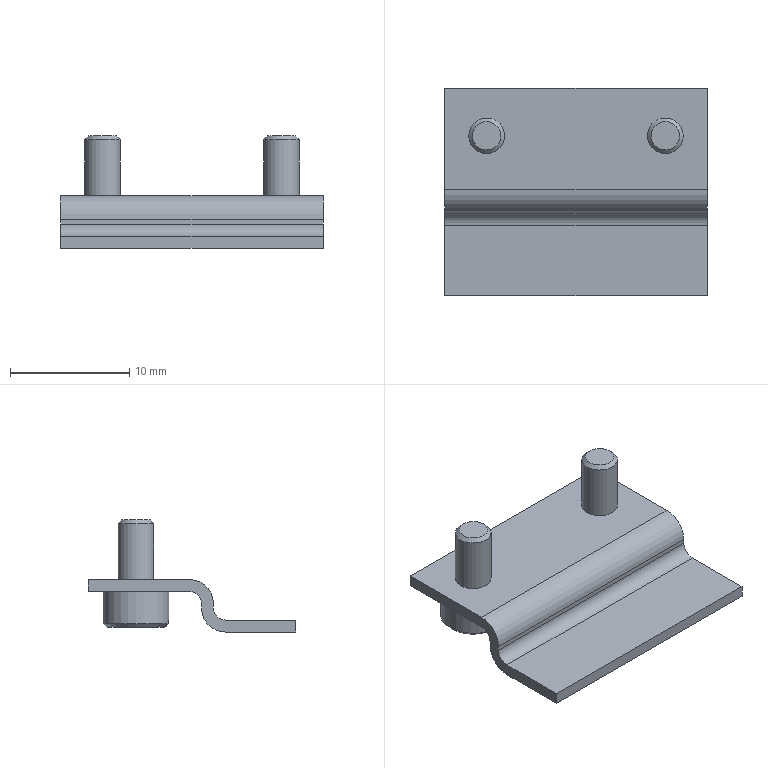Part | STEP file | LX4520CP-MX-B1-590-EP3_f | 1 solid | 40 faces | box 22 x 17.4 x 9.4 mm | volume 629.359 mm3 | plane 28 | cylinder 8 | cone 4 | commonest cylinder face diameters 2 x2 3 x2 4 x2 5.5 x2
STEP:
#1=CARTESIAN_POINT('',(-9.95,0.,-4.));
#2=VERTEX_POINT('',#1);
#3=CARTESIAN_POINT('',(-7.5,0.,-4.));
#4=DIRECTION('',(0.,0.,-1.));
#5=DIRECTION('',(-1.,0.,0.));
#6=AXIS2_PLACEMENT_3D('',#3,#4,#5);
#7=CIRCLE('',#6,2.45);
#8=EDGE_CURVE('',#2,#2,#7,.T.);
#9=ORIENTED_EDGE('',*,*,#8,.T.);
#10=EDGE_LOOP('',(#9));
#11=FACE_OUTER_BOUND('',#10,.T.);
#12=CARTESIAN_POINT('',(-6.25,0.7217,-4.));
#13=VERTEX_POINT('',#12);
#14=CARTESIAN_POINT('',(-7.5,1.443,-4.));
#15=VERTEX_POINT('',#14);
#16=CARTESIAN_POINT('',(-6.25,0.7217,-4.));
#17=DIRECTION('',(-0.866,0.5,0.));
#18=VECTOR('',#17,1000.);
#19=LINE('',#16,#18);
#20=EDGE_CURVE('',#13,#15,#19,.T.);
#21=ORIENTED_EDGE('',*,*,#20,.T.);
#22=CARTESIAN_POINT('',(-8.75,0.7217,-4.));
#23=VERTEX_POINT('',#22);
#24=CARTESIAN_POINT('',(-7.5,1.443,-4.));
#25=DIRECTION('',(-0.866,-0.5,0.));
#26=VECTOR('',#25,1000.);
#27=LINE('',#24,#26);
#28=EDGE_CURVE('',#15,#23,#27,.T.);
#29=ORIENTED_EDGE('',*,*,#28,.T.);
#30=CARTESIAN_POINT('',(-8.75,-0.7217,-4.));
#31=VERTEX_POINT('',#30);
#32=CARTESIAN_POINT('',(-8.75,0.7217,-4.));
#33=DIRECTION('',(0.,-1.,0.));
#34=VECTOR('',#33,1000.);
#35=LINE('',#32,#34);
#36=EDGE_CURVE('',#23,#31,#35,.T.);
#37=ORIENTED_EDGE('',*,*,#36,.T.);
#38=CARTESIAN_POINT('',(-7.5,-1.443,-4.));
#39=VERTEX_POINT('',#38);
#40=CARTESIAN_POINT('',(-8.75,-0.7217,-4.));
#41=DIRECTION('',(0.866,-0.5,0.));
#42=VECTOR('',#41,1000.);
#43=LINE('',#40,#42);
#44=EDGE_CURVE('',#31,#39,#43,.T.);
#45=ORIENTED_EDGE('',*,*,#44,.T.);
#46=CARTESIAN_POINT('',(-6.25,-0.7217,-4.));
#47=VERTEX_POINT('',#46);
#48=CARTESIAN_POINT('',(-7.5,-1.443,-4.));
#49=DIRECTION('',(0.866,0.5,0.));
#50=VECTOR('',#49,1000.);
#51=LINE('',#48,#50);
#52=EDGE_CURVE('',#39,#47,#51,.T.);
#53=ORIENTED_EDGE('',*,*,#52,.T.);
#54=CARTESIAN_POINT('',(-6.25,-0.7217,-4.));
#55=DIRECTION('',(0.,1.,0.));
#56=VECTOR('',#55,1000.);
#57=LINE('',#54,#56);
#58=EDGE_CURVE('',#47,#13,#57,.T.);
#59=ORIENTED_EDGE('',*,*,#58,.T.);
#60=EDGE_LOOP('',(#21,#29,#37,#45,#53,#59));
#61=FACE_BOUND('',#60,.T.);
#62=CARTESIAN_POINT('',(-7.5,2.45,-4.));
#63=DIRECTION('',(0.,0.,1.));
#64=DIRECTION('',(1.,0.,0.));
#65=AXIS2_PLACEMENT_3D('',#62,#63,#64);
#66=PLANE('',#65);
#67=ADVANCED_FACE('',(#11,#61),#66,.F.);
#68=CARTESIAN_POINT('',(5.05,0.,-4.));
#69=VERTEX_POINT('',#68);
#70=CARTESIAN_POINT('',(7.5,0.,-4.));
#71=DIRECTION('',(0.,0.,-1.));
#72=DIRECTION('',(-1.,0.,0.));
#73=AXIS2_PLACEMENT_3D('',#70,#71,#72);
#74=CIRCLE('',#73,2.45);
#75=EDGE_CURVE('',#69,#69,#74,.T.);
#76=ORIENTED_EDGE('',*,*,#75,.T.);
#77=EDGE_LOOP('',(#76));
#78=FACE_OUTER_BOUND('',#77,.T.);
#79=CARTESIAN_POINT('',(8.75,0.7217,-4.));
#80=VERTEX_POINT('',#79);
#81=CARTESIAN_POINT('',(7.5,1.443,-4.));
#82=VERTEX_POINT('',#81);
#83=CARTESIAN_POINT('',(8.75,0.7217,-4.));
#84=DIRECTION('',(-0.866,0.5,0.));
#85=VECTOR('',#84,1000.);
#86=LINE('',#83,#85);
#87=EDGE_CURVE('',#80,#82,#86,.T.);
#88=ORIENTED_EDGE('',*,*,#87,.T.);
#89=CARTESIAN_POINT('',(6.25,0.7217,-4.));
#90=VERTEX_POINT('',#89);
#91=CARTESIAN_POINT('',(7.5,1.443,-4.));
#92=DIRECTION('',(-0.866,-0.5,0.));
#93=VECTOR('',#92,1000.);
#94=LINE('',#91,#93);
#95=EDGE_CURVE('',#82,#90,#94,.T.);
#96=ORIENTED_EDGE('',*,*,#95,.T.);
#97=CARTESIAN_POINT('',(6.25,-0.7217,-4.));
#98=VERTEX_POINT('',#97);
#99=CARTESIAN_POINT('',(6.25,0.7217,-4.));
#100=DIRECTION('',(0.,-1.,0.));
#101=VECTOR('',#100,1000.);
#102=LINE('',#99,#101);
#103=EDGE_CURVE('',#90,#98,#102,.T.);
#104=ORIENTED_EDGE('',*,*,#103,.T.);
#105=CARTESIAN_POINT('',(7.5,-1.443,-4.));
#106=VERTEX_POINT('',#105);
#107=CARTESIAN_POINT('',(6.25,-0.7217,-4.));
#108=DIRECTION('',(0.866,-0.5,0.));
#109=VECTOR('',#108,1000.);
#110=LINE('',#107,#109);
#111=EDGE_CURVE('',#98,#106,#110,.T.);
#112=ORIENTED_EDGE('',*,*,#111,.T.);
#113=CARTESIAN_POINT('',(8.75,-0.7217,-4.));
#114=VERTEX_POINT('',#113);
#115=CARTESIAN_POINT('',(7.5,-1.443,-4.));
#116=DIRECTION('',(0.866,0.5,0.));
#117=VECTOR('',#116,1000.);
#118=LINE('',#115,#117);
#119=EDGE_CURVE('',#106,#114,#118,.T.);
#120=ORIENTED_EDGE('',*,*,#119,.T.);
#121=CARTESIAN_POINT('',(8.75,-0.7217,-4.));
#122=DIRECTION('',(0.,1.,0.));
#123=VECTOR('',#122,1000.);
#124=LINE('',#121,#123);
#125=EDGE_CURVE('',#114,#80,#124,.T.);
#126=ORIENTED_EDGE('',*,*,#125,.T.);
#127=EDGE_LOOP('',(#88,#96,#104,#112,#120,#126));
#128=FACE_BOUND('',#127,.T.);
#129=CARTESIAN_POINT('',(7.5,2.45,-4.));
#130=DIRECTION('',(0.,0.,1.));
#131=DIRECTION('',(1.,0.,0.));
#132=AXIS2_PLACEMENT_3D('',#129,#130,#131);
#133=PLANE('',#132);
#134=ADVANCED_FACE('',(#78,#128),#133,.F.);
#135=CARTESIAN_POINT('',(-11.,4.,-1.));
#136=VERTEX_POINT('',#135);
#137=CARTESIAN_POINT('',(-11.,4.,0.));
#138=VERTEX_POINT('',#137);
#139=CARTESIAN_POINT('',(-11.,4.,-1.));
#140=DIRECTION('',(0.,0.,1.));
#141=VECTOR('',#140,1000.);
#142=LINE('',#139,#141);
#143=EDGE_CURVE('',#136,#138,#142,.T.);
#144=ORIENTED_EDGE('',*,*,#143,.T.);
#145=CARTESIAN_POINT('',(11.,4.,0.));
#146=VERTEX_POINT('',#145);
#147=CARTESIAN_POINT('',(11.,4.,0.));
#148=DIRECTION('',(-1.,0.,0.));
#149=VECTOR('',#148,1000.);
#150=LINE('',#147,#149);
#151=EDGE_CURVE('',#146,#138,#150,.T.);
#152=ORIENTED_EDGE('',*,*,#151,.F.);
#153=CARTESIAN_POINT('',(11.,4.,-1.));
#154=VERTEX_POINT('',#153);
#155=CARTESIAN_POINT('',(11.,4.,-1.));
#156=DIRECTION('',(0.,0.,1.));
#157=VECTOR('',#156,1000.);
#158=LINE('',#155,#157);
#159=EDGE_CURVE('',#154,#146,#158,.T.);
#160=ORIENTED_EDGE('',*,*,#159,.F.);
#161=CARTESIAN_POINT('',(11.,4.,-1.));
#162=DIRECTION('',(-1.,0.,0.));
#163=VECTOR('',#162,1000.);
#164=LINE('',#161,#163);
#165=EDGE_CURVE('',#154,#136,#164,.T.);
#166=ORIENTED_EDGE('',*,*,#165,.T.);
#167=EDGE_LOOP('',(#144,#152,#160,#166));
#168=FACE_OUTER_BOUND('',#167,.T.);
#169=CARTESIAN_POINT('',(11.,4.,-1.));
#170=DIRECTION('',(0.,-1.,0.));
#171=DIRECTION('',(0.,0.,-1.));
#172=AXIS2_PLACEMENT_3D('',#169,#170,#171);
#173=PLANE('',#172);
#174=ADVANCED_FACE('',(#168),#173,.F.);
#175=CARTESIAN_POINT('',(-11.,-4.5,0.));
#176=VERTEX_POINT('',#175);
#177=CARTESIAN_POINT('',(-11.,4.,0.));
#178=DIRECTION('',(0.,-1.,0.));
#179=VECTOR('',#178,1000.);
#180=LINE('',#177,#179);
#181=EDGE_CURVE('',#138,#176,#180,.T.);
#182=ORIENTED_EDGE('',*,*,#181,.T.);
#183=CARTESIAN_POINT('',(11.,-4.5,0.));
#184=VERTEX_POINT('',#183);
#185=CARTESIAN_POINT('',(11.,-4.5,0.));
#186=DIRECTION('',(-1.,0.,0.));
#187=VECTOR('',#186,1000.);
#188=LINE('',#185,#187);
#189=EDGE_CURVE('',#184,#176,#188,.T.);
#190=ORIENTED_EDGE('',*,*,#189,.F.);
#191=CARTESIAN_POINT('',(11.,4.,0.));
#192=DIRECTION('',(0.,-1.,0.));
#193=VECTOR('',#192,1000.);
#194=LINE('',#191,#193);
#195=EDGE_CURVE('',#146,#184,#194,.T.);
#196=ORIENTED_EDGE('',*,*,#195,.F.);
#197=ORIENTED_EDGE('',*,*,#151,.T.);
#198=EDGE_LOOP('',(#182,#190,#196,#197));
#199=FACE_OUTER_BOUND('',#198,.T.);
#200=CARTESIAN_POINT('',(-9.,0.,0.));
#201=VERTEX_POINT('',#200);
#202=CARTESIAN_POINT('',(-6.,0.,0.));
#203=VERTEX_POINT('',#202);
#204=CARTESIAN_POINT('',(-7.5,0.,0.));
#205=DIRECTION('',(0.,0.,-1.));
#206=DIRECTION('',(-1.,0.,0.));
#207=AXIS2_PLACEMENT_3D('',#204,#205,#206);
#208=CIRCLE('',#207,1.5);
#209=EDGE_CURVE('',#201,#203,#208,.F.);
#210=ORIENTED_EDGE('',*,*,#209,.F.);
#211=CARTESIAN_POINT('',(-7.5,0.,0.));
#212=DIRECTION('',(0.,0.,-1.));
#213=DIRECTION('',(-1.,0.,0.));
#214=AXIS2_PLACEMENT_3D('',#211,#212,#213);
#215=CIRCLE('',#214,1.5);
#216=EDGE_CURVE('',#203,#201,#215,.F.);
#217=ORIENTED_EDGE('',*,*,#216,.F.);
#218=EDGE_LOOP('',(#210,#217));
#219=FACE_BOUND('',#218,.T.);
#220=CARTESIAN_POINT('',(6.,0.,0.));
#221=VERTEX_POINT('',#220);
#222=CARTESIAN_POINT('',(9.,0.,0.));
#223=VERTEX_POINT('',#222);
#224=CARTESIAN_POINT('',(7.5,0.,0.));
#225=DIRECTION('',(0.,0.,-1.));
#226=DIRECTION('',(-1.,0.,0.));
#227=AXIS2_PLACEMENT_3D('',#224,#225,#226);
#228=CIRCLE('',#227,1.5);
#229=EDGE_CURVE('',#221,#223,#228,.F.);
#230=ORIENTED_EDGE('',*,*,#229,.F.);
#231=CARTESIAN_POINT('',(7.5,0.,0.));
#232=DIRECTION('',(0.,0.,-1.));
#233=DIRECTION('',(-1.,0.,0.));
#234=AXIS2_PLACEMENT_3D('',#231,#232,#233);
#235=CIRCLE('',#234,1.5);
#236=EDGE_CURVE('',#223,#221,#235,.F.);
#237=ORIENTED_EDGE('',*,*,#236,.F.);
#238=EDGE_LOOP('',(#230,#237));
#239=FACE_BOUND('',#238,.T.);
#240=CARTESIAN_POINT('',(11.,4.,0.));
#241=DIRECTION('',(0.,0.,-1.));
#242=DIRECTION('',(-1.,0.,0.));
#243=AXIS2_PLACEMENT_3D('',#240,#241,#242);
#244=PLANE('',#243);
#245=ADVANCED_FACE('',(#199,#219,#239),#244,.F.);
#246=CARTESIAN_POINT('',(-11.,-6.5,-2.));
#247=VERTEX_POINT('',#246);
#248=CARTESIAN_POINT('',(-11.,-4.5,-2.));
#249=DIRECTION('',(1.,0.,0.));
#250=DIRECTION('',(0.,0.,-1.));
#251=AXIS2_PLACEMENT_3D('',#248,#249,#250);
#252=CIRCLE('',#251,2.);
#253=EDGE_CURVE('',#176,#247,#252,.T.);
#254=ORIENTED_EDGE('',*,*,#253,.T.);
#255=CARTESIAN_POINT('',(11.,-6.5,-2.));
#256=VERTEX_POINT('',#255);
#257=CARTESIAN_POINT('',(11.,-6.5,-2.));
#258=DIRECTION('',(-1.,0.,0.));
#259=VECTOR('',#258,1000.);
#260=LINE('',#257,#259);
#261=EDGE_CURVE('',#256,#247,#260,.T.);
#262=ORIENTED_EDGE('',*,*,#261,.F.);
#263=CARTESIAN_POINT('',(11.,-4.5,-2.));
#264=DIRECTION('',(1.,0.,0.));
#265=DIRECTION('',(0.,0.,-1.));
#266=AXIS2_PLACEMENT_3D('',#263,#264,#265);
#267=CIRCLE('',#266,2.);
#268=EDGE_CURVE('',#184,#256,#267,.T.);
#269=ORIENTED_EDGE('',*,*,#268,.F.);
#270=ORIENTED_EDGE('',*,*,#189,.T.);
#271=EDGE_LOOP('',(#254,#262,#269,#270));
#272=FACE_OUTER_BOUND('',#271,.T.);
#273=CARTESIAN_POINT('',(11.,-4.5,-2.));
#274=DIRECTION('',(-1.,0.,0.));
#275=DIRECTION('',(0.,0.,1.));
#276=AXIS2_PLACEMENT_3D('',#273,#274,#275);
#277=CYLINDRICAL_SURFACE('',#276,2.);
#278=ADVANCED_FACE('',(#272),#277,.T.);
#279=CARTESIAN_POINT('',(-11.,-6.5,-2.4));
#280=VERTEX_POINT('',#279);
#281=CARTESIAN_POINT('',(-11.,-6.5,-2.));
#282=DIRECTION('',(0.,0.,-1.));
#283=VECTOR('',#282,1000.);
#284=LINE('',#281,#283);
#285=EDGE_CURVE('',#247,#280,#284,.T.);
#286=ORIENTED_EDGE('',*,*,#285,.T.);
#287=CARTESIAN_POINT('',(11.,-6.5,-2.4));
#288=VERTEX_POINT('',#287);
#289=CARTESIAN_POINT('',(11.,-6.5,-2.4));
#290=DIRECTION('',(-1.,0.,0.));
#291=VECTOR('',#290,1000.);
#292=LINE('',#289,#291);
#293=EDGE_CURVE('',#288,#280,#292,.T.);
#294=ORIENTED_EDGE('',*,*,#293,.F.);
#295=CARTESIAN_POINT('',(11.,-6.5,-2.));
#296=DIRECTION('',(0.,0.,-1.));
#297=VECTOR('',#296,1000.);
#298=LINE('',#295,#297);
#299=EDGE_CURVE('',#256,#288,#298,.T.);
#300=ORIENTED_EDGE('',*,*,#299,.F.);
#301=ORIENTED_EDGE('',*,*,#261,.T.);
#302=EDGE_LOOP('',(#286,#294,#300,#301));
#303=FACE_OUTER_BOUND('',#302,.T.);
#304=CARTESIAN_POINT('',(11.,-6.5,-2.));
#305=DIRECTION('',(0.,1.,0.));
#306=DIRECTION('',(0.,0.,1.));
#307=AXIS2_PLACEMENT_3D('',#304,#305,#306);
#308=PLANE('',#307);
#309=ADVANCED_FACE('',(#303),#308,.F.);
#310=CARTESIAN_POINT('',(-11.,-7.5,-3.4));
#311=VERTEX_POINT('',#310);
#312=CARTESIAN_POINT('',(-11.,-7.5,-2.4));
#313=DIRECTION('',(1.,0.,0.));
#314=DIRECTION('',(0.,0.,-1.));
#315=AXIS2_PLACEMENT_3D('',#312,#313,#314);
#316=CIRCLE('',#315,1.);
#317=EDGE_CURVE('',#311,#280,#316,.T.);
#318=ORIENTED_EDGE('',*,*,#317,.F.);
#319=CARTESIAN_POINT('',(11.,-7.5,-3.4));
#320=VERTEX_POINT('',#319);
#321=CARTESIAN_POINT('',(11.,-7.5,-3.4));
#322=DIRECTION('',(-1.,0.,0.));
#323=VECTOR('',#322,1000.);
#324=LINE('',#321,#323);
#325=EDGE_CURVE('',#320,#311,#324,.T.);
#326=ORIENTED_EDGE('',*,*,#325,.F.);
#327=CARTESIAN_POINT('',(11.,-7.5,-2.4));
#328=DIRECTION('',(1.,0.,0.));
#329=DIRECTION('',(0.,0.,-1.));
#330=AXIS2_PLACEMENT_3D('',#327,#328,#329);
#331=CIRCLE('',#330,1.);
#332=EDGE_CURVE('',#320,#288,#331,.T.);
#333=ORIENTED_EDGE('',*,*,#332,.T.);
#334=ORIENTED_EDGE('',*,*,#293,.T.);
#335=EDGE_LOOP('',(#318,#326,#333,#334));
#336=FACE_OUTER_BOUND('',#335,.T.);
#337=CARTESIAN_POINT('',(11.,-7.5,-2.4));
#338=DIRECTION('',(-1.,0.,0.));
#339=DIRECTION('',(0.,0.,1.));
#340=AXIS2_PLACEMENT_3D('',#337,#338,#339);
#341=CYLINDRICAL_SURFACE('',#340,1.);
#342=ADVANCED_FACE('',(#336),#341,.F.);
#343=CARTESIAN_POINT('',(-11.,-13.4,-3.4));
#344=VERTEX_POINT('',#343);
#345=CARTESIAN_POINT('',(-11.,-7.5,-3.4));
#346=DIRECTION('',(0.,-1.,0.));
#347=VECTOR('',#346,1000.);
#348=LINE('',#345,#347);
#349=EDGE_CURVE('',#311,#344,#348,.T.);
#350=ORIENTED_EDGE('',*,*,#349,.T.);
#351=CARTESIAN_POINT('',(11.,-13.4,-3.4));
#352=VERTEX_POINT('',#351);
#353=CARTESIAN_POINT('',(11.,-13.4,-3.4));
#354=DIRECTION('',(-1.,0.,0.));
#355=VECTOR('',#354,1000.);
#356=LINE('',#353,#355);
#357=EDGE_CURVE('',#352,#344,#356,.T.);
#358=ORIENTED_EDGE('',*,*,#357,.F.);
#359=CARTESIAN_POINT('',(11.,-7.5,-3.4));
#360=DIRECTION('',(0.,-1.,0.));
#361=VECTOR('',#360,1000.);
#362=LINE('',#359,#361);
#363=EDGE_CURVE('',#320,#352,#362,.T.);
#364=ORIENTED_EDGE('',*,*,#363,.F.);
#365=ORIENTED_EDGE('',*,*,#325,.T.);
#366=EDGE_LOOP('',(#350,#358,#364,#365));
#367=FACE_OUTER_BOUND('',#366,.T.);
#368=CARTESIAN_POINT('',(11.,-7.5,-3.4));
#369=DIRECTION('',(0.,0.,-1.));
#370=DIRECTION('',(0.,1.,0.));
#371=AXIS2_PLACEMENT_3D('',#368,#369,#370);
#372=PLANE('',#371);
#373=ADVANCED_FACE('',(#367),#372,.F.);
#374=CARTESIAN_POINT('',(-11.,-13.4,-4.4));
#375=VERTEX_POINT('',#374);
#376=CARTESIAN_POINT('',(-11.,-13.4,-3.4));
#377=DIRECTION('',(0.,0.,-1.));
#378=VECTOR('',#377,1000.);
#379=LINE('',#376,#378);
#380=EDGE_CURVE('',#344,#375,#379,.T.);
#381=ORIENTED_EDGE('',*,*,#380,.T.);
#382=CARTESIAN_POINT('',(11.,-13.4,-4.4));
#383=VERTEX_POINT('',#382);
#384=CARTESIAN_POINT('',(11.,-13.4,-4.4));
#385=DIRECTION('',(-1.,0.,0.));
#386=VECTOR('',#385,1000.);
#387=LINE('',#384,#386);
#388=EDGE_CURVE('',#383,#375,#387,.T.);
#389=ORIENTED_EDGE('',*,*,#388,.F.);
#390=CARTESIAN_POINT('',(11.,-13.4,-3.4));
#391=DIRECTION('',(0.,0.,-1.));
#392=VECTOR('',#391,1000.);
#393=LINE('',#390,#392);
#394=EDGE_CURVE('',#352,#383,#393,.T.);
#395=ORIENTED_EDGE('',*,*,#394,.F.);
#396=ORIENTED_EDGE('',*,*,#357,.T.);
#397=EDGE_LOOP('',(#381,#389,#395,#396));
#398=FACE_OUTER_BOUND('',#397,.T.);
#399=CARTESIAN_POINT('',(11.,-13.4,-3.4));
#400=DIRECTION('',(0.,1.,0.));
#401=DIRECTION('',(0.,0.,1.));
#402=AXIS2_PLACEMENT_3D('',#399,#400,#401);
#403=PLANE('',#402);
#404=ADVANCED_FACE('',(#398),#403,.F.);
#405=CARTESIAN_POINT('',(-11.,-7.5,-4.4));
#406=VERTEX_POINT('',#405);
#407=CARTESIAN_POINT('',(-11.,-13.4,-4.4));
#408=DIRECTION('',(0.,1.,0.));
#409=VECTOR('',#408,1000.);
#410=LINE('',#407,#409);
#411=EDGE_CURVE('',#375,#406,#410,.T.);
#412=ORIENTED_EDGE('',*,*,#411,.T.);
#413=CARTESIAN_POINT('',(11.,-7.5,-4.4));
#414=VERTEX_POINT('',#413);
#415=CARTESIAN_POINT('',(11.,-7.5,-4.4));
#416=DIRECTION('',(-1.,0.,0.));
#417=VECTOR('',#416,1000.);
#418=LINE('',#415,#417);
#419=EDGE_CURVE('',#414,#406,#418,.T.);
#420=ORIENTED_EDGE('',*,*,#419,.F.);
#421=CARTESIAN_POINT('',(11.,-13.4,-4.4));
#422=DIRECTION('',(0.,1.,0.));
#423=VECTOR('',#422,1000.);
#424=LINE('',#421,#423);
#425=EDGE_CURVE('',#383,#414,#424,.T.);
#426=ORIENTED_EDGE('',*,*,#425,.F.);
#427=ORIENTED_EDGE('',*,*,#388,.T.);
#428=EDGE_LOOP('',(#412,#420,#426,#427));
#429=FACE_OUTER_BOUND('',#428,.T.);
#430=CARTESIAN_POINT('',(11.,-13.4,-4.4));
#431=DIRECTION('',(0.,0.,1.));
#432=DIRECTION('',(1.,0.,0.));
#433=AXIS2_PLACEMENT_3D('',#430,#431,#432);
#434=PLANE('',#433);
#435=ADVANCED_FACE('',(#429),#434,.F.);
#436=CARTESIAN_POINT('',(-11.,-5.5,-2.4));
#437=VERTEX_POINT('',#436);
#438=CARTESIAN_POINT('',(-11.,-7.5,-2.4));
#439=DIRECTION('',(1.,0.,0.));
#440=DIRECTION('',(0.,0.,-1.));
#441=AXIS2_PLACEMENT_3D('',#438,#439,#440);
#442=CIRCLE('',#441,2.);
#443=EDGE_CURVE('',#406,#437,#442,.T.);
#444=ORIENTED_EDGE('',*,*,#443,.T.);
#445=CARTESIAN_POINT('',(11.,-5.5,-2.4));
#446=VERTEX_POINT('',#445);
#447=CARTESIAN_POINT('',(11.,-5.5,-2.4));
#448=DIRECTION('',(-1.,0.,0.));
#449=VECTOR('',#448,1000.);
#450=LINE('',#447,#449);
#451=EDGE_CURVE('',#446,#437,#450,.T.);
#452=ORIENTED_EDGE('',*,*,#451,.F.);
#453=CARTESIAN_POINT('',(11.,-7.5,-2.4));
#454=DIRECTION('',(1.,0.,0.));
#455=DIRECTION('',(0.,0.,-1.));
#456=AXIS2_PLACEMENT_3D('',#453,#454,#455);
#457=CIRCLE('',#456,2.);
#458=EDGE_CURVE('',#414,#446,#457,.T.);
#459=ORIENTED_EDGE('',*,*,#458,.F.);
#460=ORIENTED_EDGE('',*,*,#419,.T.);
#461=EDGE_LOOP('',(#444,#452,#459,#460));
#462=FACE_OUTER_BOUND('',#461,.T.);
#463=CARTESIAN_POINT('',(11.,-7.5,-2.4));
#464=DIRECTION('',(-1.,0.,0.));
#465=DIRECTION('',(0.,0.,1.));
#466=AXIS2_PLACEMENT_3D('',#463,#464,#465);
#467=CYLINDRICAL_SURFACE('',#466,2.);
#468=ADVANCED_FACE('',(#462),#467,.T.);
#469=CARTESIAN_POINT('',(-11.,-5.5,-2.));
#470=VERTEX_POINT('',#469);
#471=CARTESIAN_POINT('',(-11.,-5.5,-2.4));
#472=DIRECTION('',(0.,0.,1.));
#473=VECTOR('',#472,1000.);
#474=LINE('',#471,#473);
#475=EDGE_CURVE('',#437,#470,#474,.T.);
#476=ORIENTED_EDGE('',*,*,#475,.T.);
#477=CARTESIAN_POINT('',(11.,-5.5,-2.));
#478=VERTEX_POINT('',#477);
#479=CARTESIAN_POINT('',(11.,-5.5,-2.));
#480=DIRECTION('',(-1.,0.,0.));
#481=VECTOR('',#480,1000.);
#482=LINE('',#479,#481);
#483=EDGE_CURVE('',#478,#470,#482,.T.);
#484=ORIENTED_EDGE('',*,*,#483,.F.);
#485=CARTESIAN_POINT('',(11.,-5.5,-2.4));
#486=DIRECTION('',(0.,0.,1.));
#487=VECTOR('',#486,1000.);
#488=LINE('',#485,#487);
#489=EDGE_CURVE('',#446,#478,#488,.T.);
#490=ORIENTED_EDGE('',*,*,#489,.F.);
#491=ORIENTED_EDGE('',*,*,#451,.T.);
#492=EDGE_LOOP('',(#476,#484,#490,#491));
#493=FACE_OUTER_BOUND('',#492,.T.);
#494=CARTESIAN_POINT('',(11.,-5.5,-2.4));
#495=DIRECTION('',(0.,-1.,0.));
#496=DIRECTION('',(0.,0.,-1.));
#497=AXIS2_PLACEMENT_3D('',#494,#495,#496);
#498=PLANE('',#497);
#499=ADVANCED_FACE('',(#493),#498,.F.);
#500=CARTESIAN_POINT('',(-11.,-4.5,-1.));
#501=VERTEX_POINT('',#500);
#502=CARTESIAN_POINT('',(-11.,-4.5,-2.));
#503=DIRECTION('',(1.,0.,0.));
#504=DIRECTION('',(0.,0.,-1.));
#505=AXIS2_PLACEMENT_3D('',#502,#503,#504);
#506=CIRCLE('',#505,1.);
#507=EDGE_CURVE('',#501,#470,#506,.T.);
#508=ORIENTED_EDGE('',*,*,#507,.F.);
#509=CARTESIAN_POINT('',(11.,-4.5,-1.));
#510=VERTEX_POINT('',#509);
#511=CARTESIAN_POINT('',(11.,-4.5,-1.));
#512=DIRECTION('',(-1.,0.,0.));
#513=VECTOR('',#512,1000.);
#514=LINE('',#511,#513);
#515=EDGE_CURVE('',#510,#501,#514,.T.);
#516=ORIENTED_EDGE('',*,*,#515,.F.);
#517=CARTESIAN_POINT('',(11.,-4.5,-2.));
#518=DIRECTION('',(1.,0.,0.));
#519=DIRECTION('',(0.,0.,-1.));
#520=AXIS2_PLACEMENT_3D('',#517,#518,#519);
#521=CIRCLE('',#520,1.);
#522=EDGE_CURVE('',#510,#478,#521,.T.);
#523=ORIENTED_EDGE('',*,*,#522,.T.);
#524=ORIENTED_EDGE('',*,*,#483,.T.);
#525=EDGE_LOOP('',(#508,#516,#523,#524));
#526=FACE_OUTER_BOUND('',#525,.T.);
#527=CARTESIAN_POINT('',(11.,-4.5,-2.));
#528=DIRECTION('',(-1.,0.,0.));
#529=DIRECTION('',(0.,0.,1.));
#530=AXIS2_PLACEMENT_3D('',#527,#528,#529);
#531=CYLINDRICAL_SURFACE('',#530,1.);
#532=ADVANCED_FACE('',(#526),#531,.F.);
#533=CARTESIAN_POINT('',(-11.,-4.5,-1.));
#534=DIRECTION('',(0.,1.,0.));
#535=VECTOR('',#534,1000.);
#536=LINE('',#533,#535);
#537=EDGE_CURVE('',#501,#136,#536,.T.);
#538=ORIENTED_EDGE('',*,*,#537,.T.);
#539=ORIENTED_EDGE('',*,*,#165,.F.);
#540=CARTESIAN_POINT('',(11.,-4.5,-1.));
#541=DIRECTION('',(0.,1.,0.));
#542=VECTOR('',#541,1000.);
#543=LINE('',#540,#542);
#544=EDGE_CURVE('',#510,#154,#543,.T.);
#545=ORIENTED_EDGE('',*,*,#544,.F.);
#546=ORIENTED_EDGE('',*,*,#515,.T.);
#547=EDGE_LOOP('',(#538,#539,#545,#546));
#548=FACE_OUTER_BOUND('',#547,.T.);
#549=CARTESIAN_POINT('',(-4.75,0.,-1.));
#550=VERTEX_POINT('',#549);
#551=CARTESIAN_POINT('',(-7.5,0.,-1.));
#552=DIRECTION('',(0.,0.,1.));
#553=DIRECTION('',(1.,0.,0.));
#554=AXIS2_PLACEMENT_3D('',#551,#552,#553);
#555=CIRCLE('',#554,2.75);
#556=EDGE_CURVE('',#550,#550,#555,.F.);
#557=ORIENTED_EDGE('',*,*,#556,.F.);
#558=EDGE_LOOP('',(#557));
#559=FACE_BOUND('',#558,.T.);
#560=CARTESIAN_POINT('',(10.25,0.,-1.));
#561=VERTEX_POINT('',#560);
#562=CARTESIAN_POINT('',(7.5,0.,-1.));
#563=DIRECTION('',(0.,0.,1.));
#564=DIRECTION('',(1.,0.,0.));
#565=AXIS2_PLACEMENT_3D('',#562,#563,#564);
#566=CIRCLE('',#565,2.75);
#567=EDGE_CURVE('',#561,#561,#566,.F.);
#568=ORIENTED_EDGE('',*,*,#567,.F.);
#569=EDGE_LOOP('',(#568));
#570=FACE_BOUND('',#569,.T.);
#571=CARTESIAN_POINT('',(11.,-4.5,-1.));
#572=DIRECTION('',(0.,0.,1.));
#573=DIRECTION('',(1.,0.,0.));
#574=AXIS2_PLACEMENT_3D('',#571,#572,#573);
#575=PLANE('',#574);
#576=ADVANCED_FACE('',(#548,#559,#570),#575,.F.);
#577=ORIENTED_EDGE('',*,*,#159,.T.);
#578=ORIENTED_EDGE('',*,*,#195,.T.);
#579=ORIENTED_EDGE('',*,*,#268,.T.);
#580=ORIENTED_EDGE('',*,*,#299,.T.);
#581=ORIENTED_EDGE('',*,*,#332,.F.);
#582=ORIENTED_EDGE('',*,*,#363,.T.);
#583=ORIENTED_EDGE('',*,*,#394,.T.);
#584=ORIENTED_EDGE('',*,*,#425,.T.);
#585=ORIENTED_EDGE('',*,*,#458,.T.);
#586=ORIENTED_EDGE('',*,*,#489,.T.);
#587=ORIENTED_EDGE('',*,*,#522,.F.);
#588=ORIENTED_EDGE('',*,*,#544,.T.);
#589=EDGE_LOOP('',(#577,#578,#579,#580,#581,#582,#583,#584,#585,#586,#587,#588));
#590=FACE_OUTER_BOUND('',#589,.T.);
#591=CARTESIAN_POINT('',(11.,-4.5,-2.));
#592=DIRECTION('',(1.,0.,0.));
#593=DIRECTION('',(0.,0.,-1.));
#594=AXIS2_PLACEMENT_3D('',#591,#592,#593);
#595=PLANE('',#594);
#596=ADVANCED_FACE('',(#590),#595,.T.);
#597=ORIENTED_EDGE('',*,*,#143,.F.);
#598=ORIENTED_EDGE('',*,*,#537,.F.);
#599=ORIENTED_EDGE('',*,*,#507,.T.);
#600=ORIENTED_EDGE('',*,*,#475,.F.);
#601=ORIENTED_EDGE('',*,*,#443,.F.);
#602=ORIENTED_EDGE('',*,*,#411,.F.);
#603=ORIENTED_EDGE('',*,*,#380,.F.);
#604=ORIENTED_EDGE('',*,*,#349,.F.);
#605=ORIENTED_EDGE('',*,*,#317,.T.);
#606=ORIENTED_EDGE('',*,*,#285,.F.);
#607=ORIENTED_EDGE('',*,*,#253,.F.);
#608=ORIENTED_EDGE('',*,*,#181,.F.);
#609=EDGE_LOOP('',(#597,#598,#599,#600,#601,#602,#603,#604,#605,#606,#607,#608));
#610=FACE_OUTER_BOUND('',#609,.T.);
#611=CARTESIAN_POINT('',(-11.,-4.5,-2.));
#612=DIRECTION('',(1.,0.,0.));
#613=DIRECTION('',(0.,0.,-1.));
#614=AXIS2_PLACEMENT_3D('',#611,#612,#613);
#615=PLANE('',#614);
#616=ADVANCED_FACE('',(#610),#615,.F.);
#617=CARTESIAN_POINT('',(4.75,0.,-3.7));
#618=VERTEX_POINT('',#617);
#619=CARTESIAN_POINT('',(10.25,0.,-3.7));
#620=VERTEX_POINT('',#619);
#621=CARTESIAN_POINT('',(7.5,0.,-3.7));
#622=DIRECTION('',(0.,0.,-1.));
#623=DIRECTION('',(-1.,0.,0.));
#624=AXIS2_PLACEMENT_3D('',#621,#622,#623);
#625=CIRCLE('',#624,2.75);
#626=EDGE_CURVE('',#618,#620,#625,.T.);
#627=ORIENTED_EDGE('',*,*,#626,.T.);
#628=CARTESIAN_POINT('',(7.5,0.,-3.7));
#629=DIRECTION('',(0.,0.,-1.));
#630=DIRECTION('',(-1.,0.,0.));
#631=AXIS2_PLACEMENT_3D('',#628,#629,#630);
#632=CIRCLE('',#631,2.75);
#633=EDGE_CURVE('',#620,#618,#632,.T.);
#634=ORIENTED_EDGE('',*,*,#633,.T.);
#635=CARTESIAN_POINT('',(4.75,0.,-3.7));
#636=DIRECTION('',(0.7071,0.,-0.7071));
#637=VECTOR('',#636,2.75);
#638=LINE('',#635,#637);
#639=EDGE_CURVE('',#618,#69,#638,.T.);
#640=ORIENTED_EDGE('',*,*,#639,.T.);
#641=ORIENTED_EDGE('',*,*,#75,.F.);
#642=ORIENTED_EDGE('',*,*,#639,.F.);
#643=EDGE_LOOP('',(#627,#634,#640,#641,#642));
#644=FACE_OUTER_BOUND('',#643,.T.);
#645=CARTESIAN_POINT('',(7.5,0.,-3.7));
#646=DIRECTION('',(0.,0.,1.));
#647=DIRECTION('',(1.,0.,0.));
#648=AXIS2_PLACEMENT_3D('',#645,#646,#647);
#649=CONICAL_SURFACE('',#648,2.75,0.7854);
#650=ADVANCED_FACE('',(#644),#649,.T.);
#651=ORIENTED_EDGE('',*,*,#626,.F.);
#652=ORIENTED_EDGE('',*,*,#633,.F.);
#653=CARTESIAN_POINT('',(10.25,0.,-4.));
#654=DIRECTION('',(0.,0.,1.));
#655=VECTOR('',#654,2.75);
#656=LINE('',#653,#655);
#657=EDGE_CURVE('',#620,#561,#656,.T.);
#658=ORIENTED_EDGE('',*,*,#657,.T.);
#659=ORIENTED_EDGE('',*,*,#567,.T.);
#660=ORIENTED_EDGE('',*,*,#657,.F.);
#661=EDGE_LOOP('',(#651,#652,#658,#659,#660));
#662=FACE_OUTER_BOUND('',#661,.T.);
#663=CARTESIAN_POINT('',(7.5,0.,-4.));
#664=DIRECTION('',(0.,0.,-1.));
#665=DIRECTION('',(-1.,0.,0.));
#666=AXIS2_PLACEMENT_3D('',#663,#664,#665);
#667=CYLINDRICAL_SURFACE('',#666,2.75);
#668=ADVANCED_FACE('',(#662),#667,.T.);
#669=ORIENTED_EDGE('',*,*,#229,.T.);
#670=CARTESIAN_POINT('',(9.,0.,4.694));
#671=VERTEX_POINT('',#670);
#672=CARTESIAN_POINT('',(9.,0.,-4.));
#673=DIRECTION('',(0.,0.,1.));
#674=VECTOR('',#673,1.5);
#675=LINE('',#672,#674);
#676=EDGE_CURVE('',#223,#671,#675,.T.);
#677=ORIENTED_EDGE('',*,*,#676,.T.);
#678=CARTESIAN_POINT('',(6.,0.,4.694));
#679=VERTEX_POINT('',#678);
#680=CARTESIAN_POINT('',(7.5,0.,4.694));
#681=DIRECTION('',(0.,0.,-1.));
#682=DIRECTION('',(-1.,0.,0.));
#683=AXIS2_PLACEMENT_3D('',#680,#681,#682);
#684=CIRCLE('',#683,1.5);
#685=EDGE_CURVE('',#671,#679,#684,.T.);
#686=ORIENTED_EDGE('',*,*,#685,.T.);
#687=CARTESIAN_POINT('',(7.5,0.,4.694));
#688=DIRECTION('',(0.,0.,-1.));
#689=DIRECTION('',(-1.,0.,0.));
#690=AXIS2_PLACEMENT_3D('',#687,#688,#689);
#691=CIRCLE('',#690,1.5);
#692=EDGE_CURVE('',#679,#671,#691,.T.);
#693=ORIENTED_EDGE('',*,*,#692,.T.);
#694=ORIENTED_EDGE('',*,*,#676,.F.);
#695=ORIENTED_EDGE('',*,*,#236,.T.);
#696=EDGE_LOOP('',(#669,#677,#686,#693,#694,#695));
#697=FACE_OUTER_BOUND('',#696,.T.);
#698=CARTESIAN_POINT('',(7.5,0.,-4.));
#699=DIRECTION('',(0.,0.,-1.));
#700=DIRECTION('',(-1.,0.,0.));
#701=AXIS2_PLACEMENT_3D('',#698,#699,#700);
#702=CYLINDRICAL_SURFACE('',#701,1.5);
#703=ADVANCED_FACE('',(#697),#702,.T.);
#704=CARTESIAN_POINT('',(6.306,0.,5.));
#705=VERTEX_POINT('',#704);
#706=CARTESIAN_POINT('',(8.694,0.,5.));
#707=VERTEX_POINT('',#706);
#708=CARTESIAN_POINT('',(7.5,0.,5.));
#709=DIRECTION('',(0.,0.,-1.));
#710=DIRECTION('',(-1.,0.,0.));
#711=AXIS2_PLACEMENT_3D('',#708,#709,#710);
#712=CIRCLE('',#711,1.194);
#713=EDGE_CURVE('',#705,#707,#712,.T.);
#714=ORIENTED_EDGE('',*,*,#713,.F.);
#715=CARTESIAN_POINT('',(7.5,0.,5.));
#716=DIRECTION('',(0.,0.,-1.));
#717=DIRECTION('',(-1.,0.,0.));
#718=AXIS2_PLACEMENT_3D('',#715,#716,#717);
#719=CIRCLE('',#718,1.194);
#720=EDGE_CURVE('',#707,#705,#719,.T.);
#721=ORIENTED_EDGE('',*,*,#720,.F.);
#722=EDGE_LOOP('',(#714,#721));
#723=FACE_OUTER_BOUND('',#722,.T.);
#724=CARTESIAN_POINT('',(7.5,0.,5.));
#725=DIRECTION('',(0.,0.,-1.));
#726=DIRECTION('',(-1.,0.,0.));
#727=AXIS2_PLACEMENT_3D('',#724,#725,#726);
#728=PLANE('',#727);
#729=ADVANCED_FACE('',(#723),#728,.F.);
#730=ORIENTED_EDGE('',*,*,#692,.F.);
#731=ORIENTED_EDGE('',*,*,#685,.F.);
#732=CARTESIAN_POINT('',(8.694,0.,5.));
#733=DIRECTION('',(-0.7071,0.,0.7071));
#734=VECTOR('',#733,1.194);
#735=LINE('',#732,#734);
#736=EDGE_CURVE('',#671,#707,#735,.T.);
#737=ORIENTED_EDGE('',*,*,#736,.T.);
#738=ORIENTED_EDGE('',*,*,#720,.T.);
#739=ORIENTED_EDGE('',*,*,#713,.T.);
#740=ORIENTED_EDGE('',*,*,#736,.F.);
#741=EDGE_LOOP('',(#730,#731,#737,#738,#739,#740));
#742=FACE_OUTER_BOUND('',#741,.T.);
#743=CARTESIAN_POINT('',(7.5,0.,5.));
#744=DIRECTION('',(0.,0.,-1.));
#745=DIRECTION('',(-1.,0.,0.));
#746=AXIS2_PLACEMENT_3D('',#743,#744,#745);
#747=CONICAL_SURFACE('',#746,1.194,0.7854);
#748=ADVANCED_FACE('',(#742),#747,.T.);
#749=CARTESIAN_POINT('',(-10.25,0.,-3.7));
#750=VERTEX_POINT('',#749);
#751=CARTESIAN_POINT('',(-4.75,0.,-3.7));
#752=VERTEX_POINT('',#751);
#753=CARTESIAN_POINT('',(-7.5,0.,-3.7));
#754=DIRECTION('',(0.,0.,-1.));
#755=DIRECTION('',(-1.,0.,0.));
#756=AXIS2_PLACEMENT_3D('',#753,#754,#755);
#757=CIRCLE('',#756,2.75);
#758=EDGE_CURVE('',#750,#752,#757,.T.);
#759=ORIENTED_EDGE('',*,*,#758,.T.);
#760=CARTESIAN_POINT('',(-7.5,0.,-3.7));
#761=DIRECTION('',(0.,0.,-1.));
#762=DIRECTION('',(-1.,0.,0.));
#763=AXIS2_PLACEMENT_3D('',#760,#761,#762);
#764=CIRCLE('',#763,2.75);
#765=EDGE_CURVE('',#752,#750,#764,.T.);
#766=ORIENTED_EDGE('',*,*,#765,.T.);
#767=CARTESIAN_POINT('',(-10.25,0.,-3.7));
#768=DIRECTION('',(0.7071,0.,-0.7071));
#769=VECTOR('',#768,2.75);
#770=LINE('',#767,#769);
#771=EDGE_CURVE('',#750,#2,#770,.T.);
#772=ORIENTED_EDGE('',*,*,#771,.T.);
#773=ORIENTED_EDGE('',*,*,#8,.F.);
#774=ORIENTED_EDGE('',*,*,#771,.F.);
#775=EDGE_LOOP('',(#759,#766,#772,#773,#774));
#776=FACE_OUTER_BOUND('',#775,.T.);
#777=CARTESIAN_POINT('',(-7.5,0.,-3.7));
#778=DIRECTION('',(0.,0.,1.));
#779=DIRECTION('',(1.,0.,0.));
#780=AXIS2_PLACEMENT_3D('',#777,#778,#779);
#781=CONICAL_SURFACE('',#780,2.75,0.7854);
#782=ADVANCED_FACE('',(#776),#781,.T.);
#783=ORIENTED_EDGE('',*,*,#758,.F.);
#784=ORIENTED_EDGE('',*,*,#765,.F.);
#785=CARTESIAN_POINT('',(-4.75,0.,-4.));
#786=DIRECTION('',(0.,0.,1.));
#787=VECTOR('',#786,2.75);
#788=LINE('',#785,#787);
#789=EDGE_CURVE('',#752,#550,#788,.T.);
#790=ORIENTED_EDGE('',*,*,#789,.T.);
#791=ORIENTED_EDGE('',*,*,#556,.T.);
#792=ORIENTED_EDGE('',*,*,#789,.F.);
#793=EDGE_LOOP('',(#783,#784,#790,#791,#792));
#794=FACE_OUTER_BOUND('',#793,.T.);
#795=CARTESIAN_POINT('',(-7.5,0.,-4.));
#796=DIRECTION('',(0.,0.,-1.));
#797=DIRECTION('',(-1.,0.,0.));
#798=AXIS2_PLACEMENT_3D('',#795,#796,#797);
#799=CYLINDRICAL_SURFACE('',#798,2.75);
#800=ADVANCED_FACE('',(#794),#799,.T.);
#801=ORIENTED_EDGE('',*,*,#209,.T.);
#802=CARTESIAN_POINT('',(-6.,0.,4.694));
#803=VERTEX_POINT('',#802);
#804=CARTESIAN_POINT('',(-6.,0.,-4.));
#805=DIRECTION('',(0.,0.,1.));
#806=VECTOR('',#805,1.5);
#807=LINE('',#804,#806);
#808=EDGE_CURVE('',#203,#803,#807,.T.);
#809=ORIENTED_EDGE('',*,*,#808,.T.);
#810=CARTESIAN_POINT('',(-9.,0.,4.694));
#811=VERTEX_POINT('',#810);
#812=CARTESIAN_POINT('',(-7.5,0.,4.694));
#813=DIRECTION('',(0.,0.,-1.));
#814=DIRECTION('',(-1.,0.,0.));
#815=AXIS2_PLACEMENT_3D('',#812,#813,#814);
#816=CIRCLE('',#815,1.5);
#817=EDGE_CURVE('',#803,#811,#816,.T.);
#818=ORIENTED_EDGE('',*,*,#817,.T.);
#819=CARTESIAN_POINT('',(-7.5,0.,4.694));
#820=DIRECTION('',(0.,0.,-1.));
#821=DIRECTION('',(-1.,0.,0.));
#822=AXIS2_PLACEMENT_3D('',#819,#820,#821);
#823=CIRCLE('',#822,1.5);
#824=EDGE_CURVE('',#811,#803,#823,.T.);
#825=ORIENTED_EDGE('',*,*,#824,.T.);
#826=ORIENTED_EDGE('',*,*,#808,.F.);
#827=ORIENTED_EDGE('',*,*,#216,.T.);
#828=EDGE_LOOP('',(#801,#809,#818,#825,#826,#827));
#829=FACE_OUTER_BOUND('',#828,.T.);
#830=CARTESIAN_POINT('',(-7.5,0.,-4.));
#831=DIRECTION('',(0.,0.,-1.));
#832=DIRECTION('',(-1.,0.,0.));
#833=AXIS2_PLACEMENT_3D('',#830,#831,#832);
#834=CYLINDRICAL_SURFACE('',#833,1.5);
#835=ADVANCED_FACE('',(#829),#834,.T.);
#836=CARTESIAN_POINT('',(-8.694,0.,5.));
#837=VERTEX_POINT('',#836);
#838=CARTESIAN_POINT('',(-6.306,0.,5.));
#839=VERTEX_POINT('',#838);
#840=CARTESIAN_POINT('',(-7.5,0.,5.));
#841=DIRECTION('',(0.,0.,-1.));
#842=DIRECTION('',(-1.,0.,0.));
#843=AXIS2_PLACEMENT_3D('',#840,#841,#842);
#844=CIRCLE('',#843,1.194);
#845=EDGE_CURVE('',#837,#839,#844,.T.);
#846=ORIENTED_EDGE('',*,*,#845,.F.);
#847=CARTESIAN_POINT('',(-7.5,0.,5.));
#848=DIRECTION('',(0.,0.,-1.));
#849=DIRECTION('',(-1.,0.,0.));
#850=AXIS2_PLACEMENT_3D('',#847,#848,#849);
#851=CIRCLE('',#850,1.194);
#852=EDGE_CURVE('',#839,#837,#851,.T.);
#853=ORIENTED_EDGE('',*,*,#852,.F.);
#854=EDGE_LOOP('',(#846,#853));
#855=FACE_OUTER_BOUND('',#854,.T.);
#856=CARTESIAN_POINT('',(-7.5,0.,5.));
#857=DIRECTION('',(0.,0.,-1.));
#858=DIRECTION('',(-1.,0.,0.));
#859=AXIS2_PLACEMENT_3D('',#856,#857,#858);
#860=PLANE('',#859);
#861=ADVANCED_FACE('',(#855),#860,.F.);
#862=ORIENTED_EDGE('',*,*,#824,.F.);
#863=ORIENTED_EDGE('',*,*,#817,.F.);
#864=CARTESIAN_POINT('',(-6.306,0.,5.));
#865=DIRECTION('',(-0.7071,0.,0.7071));
#866=VECTOR('',#865,1.194);
#867=LINE('',#864,#866);
#868=EDGE_CURVE('',#803,#839,#867,.T.);
#869=ORIENTED_EDGE('',*,*,#868,.T.);
#870=ORIENTED_EDGE('',*,*,#852,.T.);
#871=ORIENTED_EDGE('',*,*,#845,.T.);
#872=ORIENTED_EDGE('',*,*,#868,.F.);
#873=EDGE_LOOP('',(#862,#863,#869,#870,#871,#872));
#874=FACE_OUTER_BOUND('',#873,.T.);
#875=CARTESIAN_POINT('',(-7.5,0.,5.));
#876=DIRECTION('',(0.,0.,-1.));
#877=DIRECTION('',(-1.,0.,0.));
#878=AXIS2_PLACEMENT_3D('',#875,#876,#877);
#879=CONICAL_SURFACE('',#878,1.194,0.7854);
#880=ADVANCED_FACE('',(#874),#879,.T.);
#881=ORIENTED_EDGE('',*,*,#103,.F.);
#882=CARTESIAN_POINT('',(6.25,0.7217,-3.));
#883=VERTEX_POINT('',#882);
#884=CARTESIAN_POINT('',(6.25,0.7217,-3.));
#885=DIRECTION('',(0.,0.,-1.));
#886=VECTOR('',#885,1000.);
#887=LINE('',#884,#886);
#888=EDGE_CURVE('',#883,#90,#887,.T.);
#889=ORIENTED_EDGE('',*,*,#888,.F.);
#890=CARTESIAN_POINT('',(6.25,-0.7217,-3.));
#891=VERTEX_POINT('',#890);
#892=CARTESIAN_POINT('',(6.25,0.7217,-3.));
#893=DIRECTION('',(0.,-1.,0.));
#894=VECTOR('',#893,1000.);
#895=LINE('',#892,#894);
#896=EDGE_CURVE('',#883,#891,#895,.T.);
#897=ORIENTED_EDGE('',*,*,#896,.T.);
#898=CARTESIAN_POINT('',(6.25,-0.7217,-3.));
#899=DIRECTION('',(0.,0.,-1.));
#900=VECTOR('',#899,1000.);
#901=LINE('',#898,#900);
#902=EDGE_CURVE('',#891,#98,#901,.T.);
#903=ORIENTED_EDGE('',*,*,#902,.T.);
#904=EDGE_LOOP('',(#881,#889,#897,#903));
#905=FACE_OUTER_BOUND('',#904,.T.);
#906=CARTESIAN_POINT('',(6.25,0.7217,-3.));
#907=DIRECTION('',(1.,0.,0.));
#908=DIRECTION('',(0.,0.,-1.));
#909=AXIS2_PLACEMENT_3D('',#906,#907,#908);
#910=PLANE('',#909);
#911=ADVANCED_FACE('',(#905),#910,.T.);
#912=ORIENTED_EDGE('',*,*,#111,.F.);
#913=ORIENTED_EDGE('',*,*,#902,.F.);
#914=CARTESIAN_POINT('',(7.5,-1.443,-3.));
#915=VERTEX_POINT('',#914);
#916=CARTESIAN_POINT('',(6.25,-0.7217,-3.));
#917=DIRECTION('',(0.866,-0.5,0.));
#918=VECTOR('',#917,1000.);
#919=LINE('',#916,#918);
#920=EDGE_CURVE('',#891,#915,#919,.T.);
#921=ORIENTED_EDGE('',*,*,#920,.T.);
#922=CARTESIAN_POINT('',(7.5,-1.443,-3.));
#923=DIRECTION('',(0.,0.,-1.));
#924=VECTOR('',#923,1000.);
#925=LINE('',#922,#924);
#926=EDGE_CURVE('',#915,#106,#925,.T.);
#927=ORIENTED_EDGE('',*,*,#926,.T.);
#928=EDGE_LOOP('',(#912,#913,#921,#927));
#929=FACE_OUTER_BOUND('',#928,.T.);
#930=CARTESIAN_POINT('',(6.25,-0.7217,-3.));
#931=DIRECTION('',(0.5,0.866,0.));
#932=DIRECTION('',(-0.866,0.5,0.));
#933=AXIS2_PLACEMENT_3D('',#930,#931,#932);
#934=PLANE('',#933);
#935=ADVANCED_FACE('',(#929),#934,.T.);
#936=ORIENTED_EDGE('',*,*,#119,.F.);
#937=ORIENTED_EDGE('',*,*,#926,.F.);
#938=CARTESIAN_POINT('',(8.75,-0.7217,-3.));
#939=VERTEX_POINT('',#938);
#940=CARTESIAN_POINT('',(7.5,-1.443,-3.));
#941=DIRECTION('',(0.866,0.5,0.));
#942=VECTOR('',#941,1000.);
#943=LINE('',#940,#942);
#944=EDGE_CURVE('',#915,#939,#943,.T.);
#945=ORIENTED_EDGE('',*,*,#944,.T.);
#946=CARTESIAN_POINT('',(8.75,-0.7217,-3.));
#947=DIRECTION('',(0.,0.,-1.));
#948=VECTOR('',#947,1000.);
#949=LINE('',#946,#948);
#950=EDGE_CURVE('',#939,#114,#949,.T.);
#951=ORIENTED_EDGE('',*,*,#950,.T.);
#952=EDGE_LOOP('',(#936,#937,#945,#951));
#953=FACE_OUTER_BOUND('',#952,.T.);
#954=CARTESIAN_POINT('',(7.5,-1.443,-3.));
#955=DIRECTION('',(-0.5,0.866,0.));
#956=DIRECTION('',(-0.866,-0.5,0.));
#957=AXIS2_PLACEMENT_3D('',#954,#955,#956);
#958=PLANE('',#957);
#959=ADVANCED_FACE('',(#953),#958,.T.);
#960=ORIENTED_EDGE('',*,*,#125,.F.);
#961=ORIENTED_EDGE('',*,*,#950,.F.);
#962=CARTESIAN_POINT('',(8.75,0.7217,-3.));
#963=VERTEX_POINT('',#962);
#964=CARTESIAN_POINT('',(8.75,-0.7217,-3.));
#965=DIRECTION('',(0.,1.,0.));
#966=VECTOR('',#965,1000.);
#967=LINE('',#964,#966);
#968=EDGE_CURVE('',#939,#963,#967,.T.);
#969=ORIENTED_EDGE('',*,*,#968,.T.);
#970=CARTESIAN_POINT('',(8.75,0.7217,-3.));
#971=DIRECTION('',(0.,0.,-1.));
#972=VECTOR('',#971,1000.);
#973=LINE('',#970,#972);
#974=EDGE_CURVE('',#963,#80,#973,.T.);
#975=ORIENTED_EDGE('',*,*,#974,.T.);
#976=EDGE_LOOP('',(#960,#961,#969,#975));
#977=FACE_OUTER_BOUND('',#976,.T.);
#978=CARTESIAN_POINT('',(8.75,-0.7217,-3.));
#979=DIRECTION('',(-1.,0.,0.));
#980=DIRECTION('',(0.,0.,1.));
#981=AXIS2_PLACEMENT_3D('',#978,#979,#980);
#982=PLANE('',#981);
#983=ADVANCED_FACE('',(#977),#982,.T.);
#984=ORIENTED_EDGE('',*,*,#87,.F.);
#985=ORIENTED_EDGE('',*,*,#974,.F.);
#986=CARTESIAN_POINT('',(7.5,1.443,-3.));
#987=VERTEX_POINT('',#986);
#988=CARTESIAN_POINT('',(8.75,0.7217,-3.));
#989=DIRECTION('',(-0.866,0.5,0.));
#990=VECTOR('',#989,1000.);
#991=LINE('',#988,#990);
#992=EDGE_CURVE('',#963,#987,#991,.T.);
#993=ORIENTED_EDGE('',*,*,#992,.T.);
#994=CARTESIAN_POINT('',(7.5,1.443,-3.));
#995=DIRECTION('',(0.,0.,-1.));
#996=VECTOR('',#995,1000.);
#997=LINE('',#994,#996);
#998=EDGE_CURVE('',#987,#82,#997,.T.);
#999=ORIENTED_EDGE('',*,*,#998,.T.);
#1000=EDGE_LOOP('',(#984,#985,#993,#999));
#1001=FACE_OUTER_BOUND('',#1000,.T.);
#1002=CARTESIAN_POINT('',(8.75,0.7217,-3.));
#1003=DIRECTION('',(-0.5,-0.866,0.));
#1004=DIRECTION('',(0.866,-0.5,0.));
#1005=AXIS2_PLACEMENT_3D('',#1002,#1003,#1004);
#1006=PLANE('',#1005);
#1007=ADVANCED_FACE('',(#1001),#1006,.T.);
#1008=ORIENTED_EDGE('',*,*,#95,.F.);
#1009=ORIENTED_EDGE('',*,*,#998,.F.);
#1010=CARTESIAN_POINT('',(7.5,1.443,-3.));
#1011=DIRECTION('',(-0.866,-0.5,0.));
#1012=VECTOR('',#1011,1000.);
#1013=LINE('',#1010,#1012);
#1014=EDGE_CURVE('',#987,#883,#1013,.T.);
#1015=ORIENTED_EDGE('',*,*,#1014,.T.);
#1016=ORIENTED_EDGE('',*,*,#888,.T.);
#1017=EDGE_LOOP('',(#1008,#1009,#1015,#1016));
#1018=FACE_OUTER_BOUND('',#1017,.T.);
#1019=CARTESIAN_POINT('',(7.5,1.443,-3.));
#1020=DIRECTION('',(0.5,-0.866,0.));
#1021=DIRECTION('',(0.866,0.5,0.));
#1022=AXIS2_PLACEMENT_3D('',#1019,#1020,#1021);
#1023=PLANE('',#1022);
#1024=ADVANCED_FACE('',(#1018),#1023,.T.);
#1025=ORIENTED_EDGE('',*,*,#896,.F.);
#1026=ORIENTED_EDGE('',*,*,#1014,.F.);
#1027=ORIENTED_EDGE('',*,*,#992,.F.);
#1028=ORIENTED_EDGE('',*,*,#968,.F.);
#1029=ORIENTED_EDGE('',*,*,#944,.F.);
#1030=ORIENTED_EDGE('',*,*,#920,.F.);
#1031=EDGE_LOOP('',(#1025,#1026,#1027,#1028,#1029,#1030));
#1032=FACE_OUTER_BOUND('',#1031,.T.);
#1033=CARTESIAN_POINT('',(0.,0.,-3.));
#1034=DIRECTION('',(0.,0.,1.));
#1035=DIRECTION('',(1.,0.,0.));
#1036=AXIS2_PLACEMENT_3D('',#1033,#1034,#1035);
#1037=PLANE('',#1036);
#1038=ADVANCED_FACE('',(#1032),#1037,.F.);
#1039=ORIENTED_EDGE('',*,*,#36,.F.);
#1040=CARTESIAN_POINT('',(-8.75,0.7217,-3.));
#1041=VERTEX_POINT('',#1040);
#1042=CARTESIAN_POINT('',(-8.75,0.7217,-3.));
#1043=DIRECTION('',(0.,0.,-1.));
#1044=VECTOR('',#1043,1000.);
#1045=LINE('',#1042,#1044);
#1046=EDGE_CURVE('',#1041,#23,#1045,.T.);
#1047=ORIENTED_EDGE('',*,*,#1046,.F.);
#1048=CARTESIAN_POINT('',(-8.75,-0.7217,-3.));
#1049=VERTEX_POINT('',#1048);
#1050=CARTESIAN_POINT('',(-8.75,0.7217,-3.));
#1051=DIRECTION('',(0.,-1.,0.));
#1052=VECTOR('',#1051,1000.);
#1053=LINE('',#1050,#1052);
#1054=EDGE_CURVE('',#1041,#1049,#1053,.T.);
#1055=ORIENTED_EDGE('',*,*,#1054,.T.);
#1056=CARTESIAN_POINT('',(-8.75,-0.7217,-3.));
#1057=DIRECTION('',(0.,0.,-1.));
#1058=VECTOR('',#1057,1000.);
#1059=LINE('',#1056,#1058);
#1060=EDGE_CURVE('',#1049,#31,#1059,.T.);
#1061=ORIENTED_EDGE('',*,*,#1060,.T.);
#1062=EDGE_LOOP('',(#1039,#1047,#1055,#1061));
#1063=FACE_OUTER_BOUND('',#1062,.T.);
#1064=CARTESIAN_POINT('',(-8.75,0.7217,-3.));
#1065=DIRECTION('',(1.,0.,0.));
#1066=DIRECTION('',(0.,0.,-1.));
#1067=AXIS2_PLACEMENT_3D('',#1064,#1065,#1066);
#1068=PLANE('',#1067);
#1069=ADVANCED_FACE('',(#1063),#1068,.T.);
#1070=ORIENTED_EDGE('',*,*,#44,.F.);
#1071=ORIENTED_EDGE('',*,*,#1060,.F.);
#1072=CARTESIAN_POINT('',(-7.5,-1.443,-3.));
#1073=VERTEX_POINT('',#1072);
#1074=CARTESIAN_POINT('',(-8.75,-0.7217,-3.));
#1075=DIRECTION('',(0.866,-0.5,0.));
#1076=VECTOR('',#1075,1000.);
#1077=LINE('',#1074,#1076);
#1078=EDGE_CURVE('',#1049,#1073,#1077,.T.);
#1079=ORIENTED_EDGE('',*,*,#1078,.T.);
#1080=CARTESIAN_POINT('',(-7.5,-1.443,-3.));
#1081=DIRECTION('',(0.,0.,-1.));
#1082=VECTOR('',#1081,1000.);
#1083=LINE('',#1080,#1082);
#1084=EDGE_CURVE('',#1073,#39,#1083,.T.);
#1085=ORIENTED_EDGE('',*,*,#1084,.T.);
#1086=EDGE_LOOP('',(#1070,#1071,#1079,#1085));
#1087=FACE_OUTER_BOUND('',#1086,.T.);
#1088=CARTESIAN_POINT('',(-8.75,-0.7217,-3.));
#1089=DIRECTION('',(0.5,0.866,0.));
#1090=DIRECTION('',(-0.866,0.5,0.));
#1091=AXIS2_PLACEMENT_3D('',#1088,#1089,#1090);
#1092=PLANE('',#1091);
#1093=ADVANCED_FACE('',(#1087),#1092,.T.);
#1094=ORIENTED_EDGE('',*,*,#52,.F.);
#1095=ORIENTED_EDGE('',*,*,#1084,.F.);
#1096=CARTESIAN_POINT('',(-6.25,-0.7217,-3.));
#1097=VERTEX_POINT('',#1096);
#1098=CARTESIAN_POINT('',(-7.5,-1.443,-3.));
#1099=DIRECTION('',(0.866,0.5,0.));
#1100=VECTOR('',#1099,1000.);
#1101=LINE('',#1098,#1100);
#1102=EDGE_CURVE('',#1073,#1097,#1101,.T.);
#1103=ORIENTED_EDGE('',*,*,#1102,.T.);
#1104=CARTESIAN_POINT('',(-6.25,-0.7217,-3.));
#1105=DIRECTION('',(0.,0.,-1.));
#1106=VECTOR('',#1105,1000.);
#1107=LINE('',#1104,#1106);
#1108=EDGE_CURVE('',#1097,#47,#1107,.T.);
#1109=ORIENTED_EDGE('',*,*,#1108,.T.);
#1110=EDGE_LOOP('',(#1094,#1095,#1103,#1109));
#1111=FACE_OUTER_BOUND('',#1110,.T.);
#1112=CARTESIAN_POINT('',(-7.5,-1.443,-3.));
#1113=DIRECTION('',(-0.5,0.866,0.));
#1114=DIRECTION('',(-0.866,-0.5,0.));
#1115=AXIS2_PLACEMENT_3D('',#1112,#1113,#1114);
#1116=PLANE('',#1115);
#1117=ADVANCED_FACE('',(#1111),#1116,.T.);
#1118=ORIENTED_EDGE('',*,*,#58,.F.);
#1119=ORIENTED_EDGE('',*,*,#1108,.F.);
#1120=CARTESIAN_POINT('',(-6.25,0.7217,-3.));
#1121=VERTEX_POINT('',#1120);
#1122=CARTESIAN_POINT('',(-6.25,-0.7217,-3.));
#1123=DIRECTION('',(0.,1.,0.));
#1124=VECTOR('',#1123,1000.);
#1125=LINE('',#1122,#1124);
#1126=EDGE_CURVE('',#1097,#1121,#1125,.T.);
#1127=ORIENTED_EDGE('',*,*,#1126,.T.);
#1128=CARTESIAN_POINT('',(-6.25,0.7217,-3.));
#1129=DIRECTION('',(0.,0.,-1.));
#1130=VECTOR('',#1129,1000.);
#1131=LINE('',#1128,#1130);
#1132=EDGE_CURVE('',#1121,#13,#1131,.T.);
#1133=ORIENTED_EDGE('',*,*,#1132,.T.);
#1134=EDGE_LOOP('',(#1118,#1119,#1127,#1133));
#1135=FACE_OUTER_BOUND('',#1134,.T.);
#1136=CARTESIAN_POINT('',(-6.25,-0.7217,-3.));
#1137=DIRECTION('',(-1.,0.,0.));
#1138=DIRECTION('',(0.,0.,1.));
#1139=AXIS2_PLACEMENT_3D('',#1136,#1137,#1138);
#1140=PLANE('',#1139);
#1141=ADVANCED_FACE('',(#1135),#1140,.T.);
#1142=ORIENTED_EDGE('',*,*,#20,.F.);
#1143=ORIENTED_EDGE('',*,*,#1132,.F.);
#1144=CARTESIAN_POINT('',(-7.5,1.443,-3.));
#1145=VERTEX_POINT('',#1144);
#1146=CARTESIAN_POINT('',(-6.25,0.7217,-3.));
#1147=DIRECTION('',(-0.866,0.5,0.));
#1148=VECTOR('',#1147,1000.);
#1149=LINE('',#1146,#1148);
#1150=EDGE_CURVE('',#1121,#1145,#1149,.T.);
#1151=ORIENTED_EDGE('',*,*,#1150,.T.);
#1152=CARTESIAN_POINT('',(-7.5,1.443,-3.));
#1153=DIRECTION('',(0.,0.,-1.));
#1154=VECTOR('',#1153,1000.);
#1155=LINE('',#1152,#1154);
#1156=EDGE_CURVE('',#1145,#15,#1155,.T.);
#1157=ORIENTED_EDGE('',*,*,#1156,.T.);
#1158=EDGE_LOOP('',(#1142,#1143,#1151,#1157));
#1159=FACE_OUTER_BOUND('',#1158,.T.);
#1160=CARTESIAN_POINT('',(-6.25,0.7217,-3.));
#1161=DIRECTION('',(-0.5,-0.866,0.));
#1162=DIRECTION('',(0.866,-0.5,0.));
#1163=AXIS2_PLACEMENT_3D('',#1160,#1161,#1162);
#1164=PLANE('',#1163);
#1165=ADVANCED_FACE('',(#1159),#1164,.T.);
#1166=ORIENTED_EDGE('',*,*,#28,.F.);
#1167=ORIENTED_EDGE('',*,*,#1156,.F.);
#1168=CARTESIAN_POINT('',(-7.5,1.443,-3.));
#1169=DIRECTION('',(-0.866,-0.5,0.));
#1170=VECTOR('',#1169,1000.);
#1171=LINE('',#1168,#1170);
#1172=EDGE_CURVE('',#1145,#1041,#1171,.T.);
#1173=ORIENTED_EDGE('',*,*,#1172,.T.);
#1174=ORIENTED_EDGE('',*,*,#1046,.T.);
#1175=EDGE_LOOP('',(#1166,#1167,#1173,#1174));
#1176=FACE_OUTER_BOUND('',#1175,.T.);
#1177=CARTESIAN_POINT('',(-7.5,1.443,-3.));
#1178=DIRECTION('',(0.5,-0.866,0.));
#1179=DIRECTION('',(0.866,0.5,0.));
#1180=AXIS2_PLACEMENT_3D('',#1177,#1178,#1179);
#1181=PLANE('',#1180);
#1182=ADVANCED_FACE('',(#1176),#1181,.T.);
#1183=ORIENTED_EDGE('',*,*,#1054,.F.);
#1184=ORIENTED_EDGE('',*,*,#1172,.F.);
#1185=ORIENTED_EDGE('',*,*,#1150,.F.);
#1186=ORIENTED_EDGE('',*,*,#1126,.F.);
#1187=ORIENTED_EDGE('',*,*,#1102,.F.);
#1188=ORIENTED_EDGE('',*,*,#1078,.F.);
#1189=EDGE_LOOP('',(#1183,#1184,#1185,#1186,#1187,#1188));
#1190=FACE_OUTER_BOUND('',#1189,.T.);
#1191=CARTESIAN_POINT('',(-15.,0.,-3.));
#1192=DIRECTION('',(0.,0.,1.));
#1193=DIRECTION('',(1.,0.,0.));
#1194=AXIS2_PLACEMENT_3D('',#1191,#1192,#1193);
#1195=PLANE('',#1194);
#1196=ADVANCED_FACE('',(#1190),#1195,.F.);
#1197=CLOSED_SHELL('',(#67,#134,#174,#245,#278,#309,#342,#373,#404,#435,#468,#499,#532,#576,#596,#616,#650,#668,#703,#729,#748,#782,#800,#835,#861,#880,#911,#935,#959,#983,#1007,#1024,#1038,#1069,#1093,#1117,#1141,#1165,#1182,#1196));
#1198=MANIFOLD_SOLID_BREP('',#1197);
#1199=(LENGTH_UNIT()NAMED_UNIT(*)SI_UNIT(.MILLI.,.METRE.));
#1200=UNCERTAINTY_MEASURE_WITH_UNIT(LENGTH_MEASURE(0.01),#1199,'','');
#1201=(NAMED_UNIT(*)PLANE_ANGLE_UNIT()SI_UNIT($,.RADIAN.));
#1202=(NAMED_UNIT(*)SI_UNIT($,.STERADIAN.)SOLID_ANGLE_UNIT());
#1203=(GEOMETRIC_REPRESENTATION_CONTEXT(3)GLOBAL_UNCERTAINTY_ASSIGNED_CONTEXT((#1200))GLOBAL_UNIT_ASSIGNED_CONTEXT((#1199,#1201,#1202))REPRESENTATION_CONTEXT('',''));
#1204=ADVANCED_BREP_SHAPE_REPRESENTATION('',(#1198),#1203);